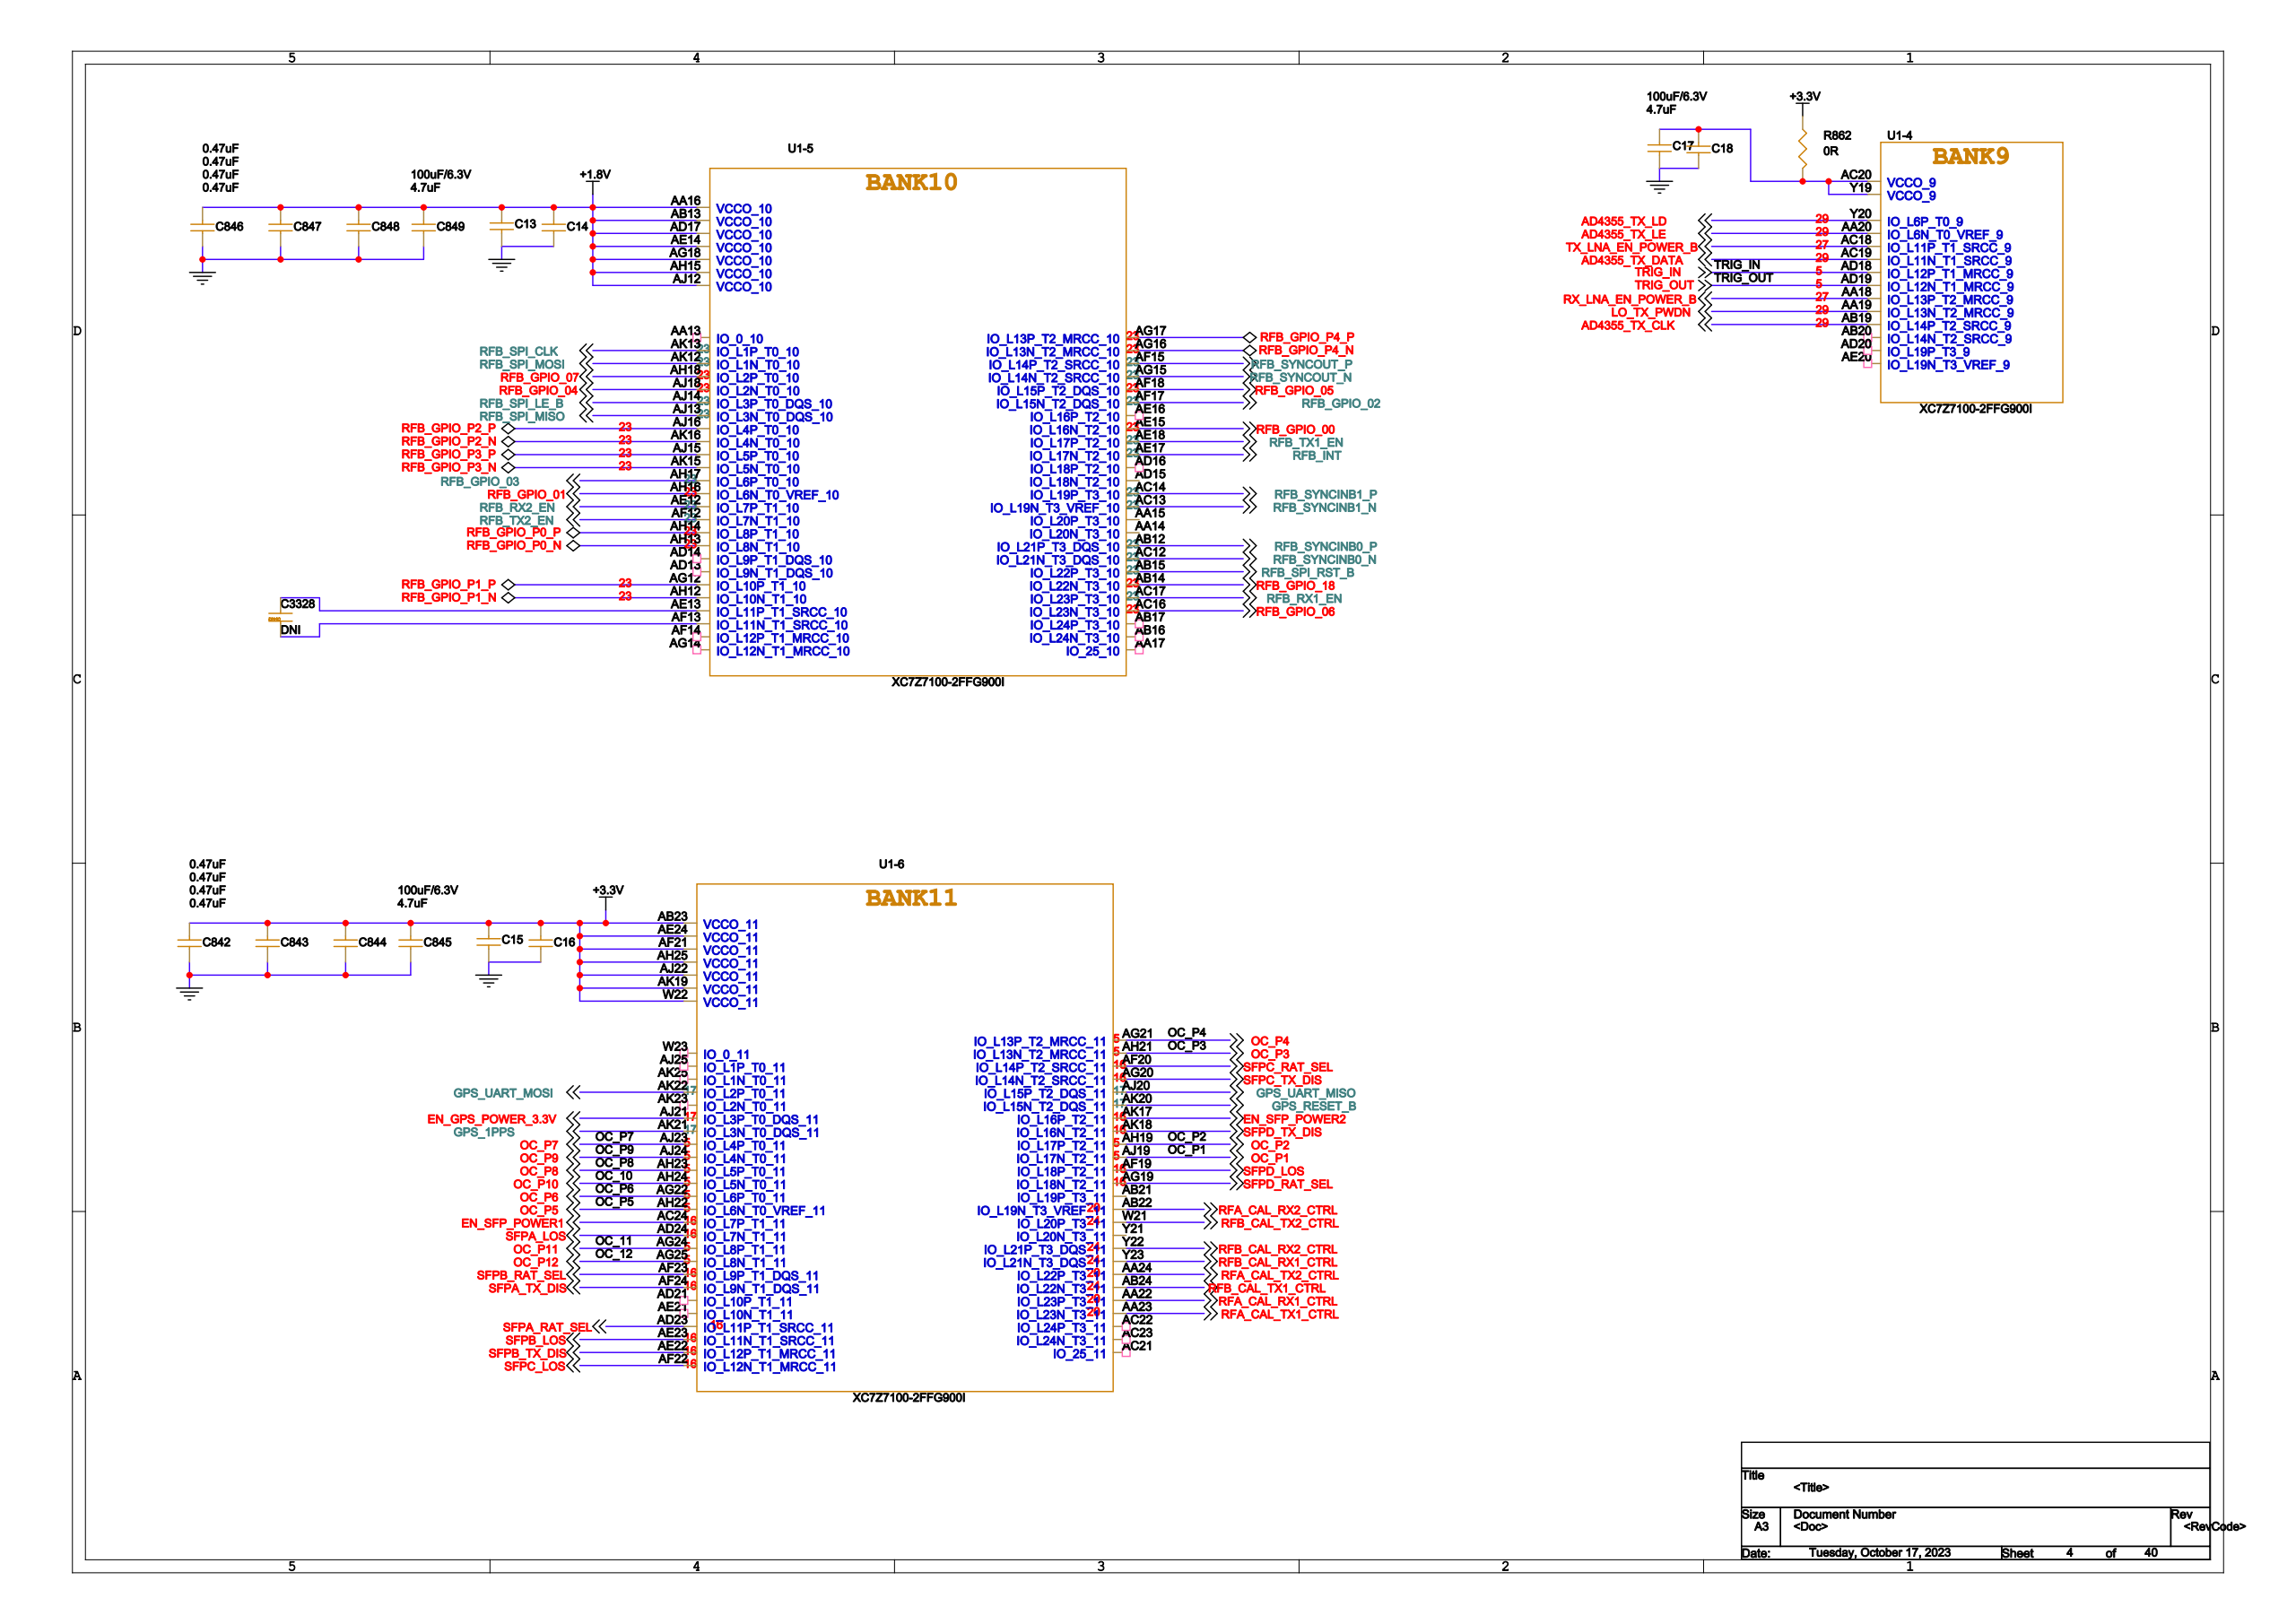Circuit board | Cadence Allegro | 1793 parts | 1223 nets | one sheet of the schematic
Parts on this sheet (reference | value | footprint):
C13 | 100uF/6.3V | 1206
C15 | 100uF/6.3V | 1206
C16 | 4.7uF | C0402
C17 | 100uF/6.3V | 1206
C842 | 0.47uF | C0402
C843 | 0.47uF | C0402
C844 | 0.47uF | C0402
C845 | 0.47uF | C0402
C846 | 0.47uF | C0402
C847 | 0.47uF | C0402
C848 | 0.47uF | C0402
C849 | 0.47uF | C0402
C3328 | DNI | C0402
R862 | 0R | R0402
Nets of these parts (net: part-pin ...):
GND: C13-2 C15-2 C16-1 C17-2 C842-1 C843-1 C844-1 C845-1 C846-1 C847-1 C848-1 C849-1
+3.3V: C15-1 C16-2 C842-2 C843-2 C844-2 C845-2 R862-2
+1.8V: C13-1 C846-2 C847-2 C848-2 C849-2
N18494: C17-1 R862-1
N17939632: C3328-1
N17939616: C3328-2